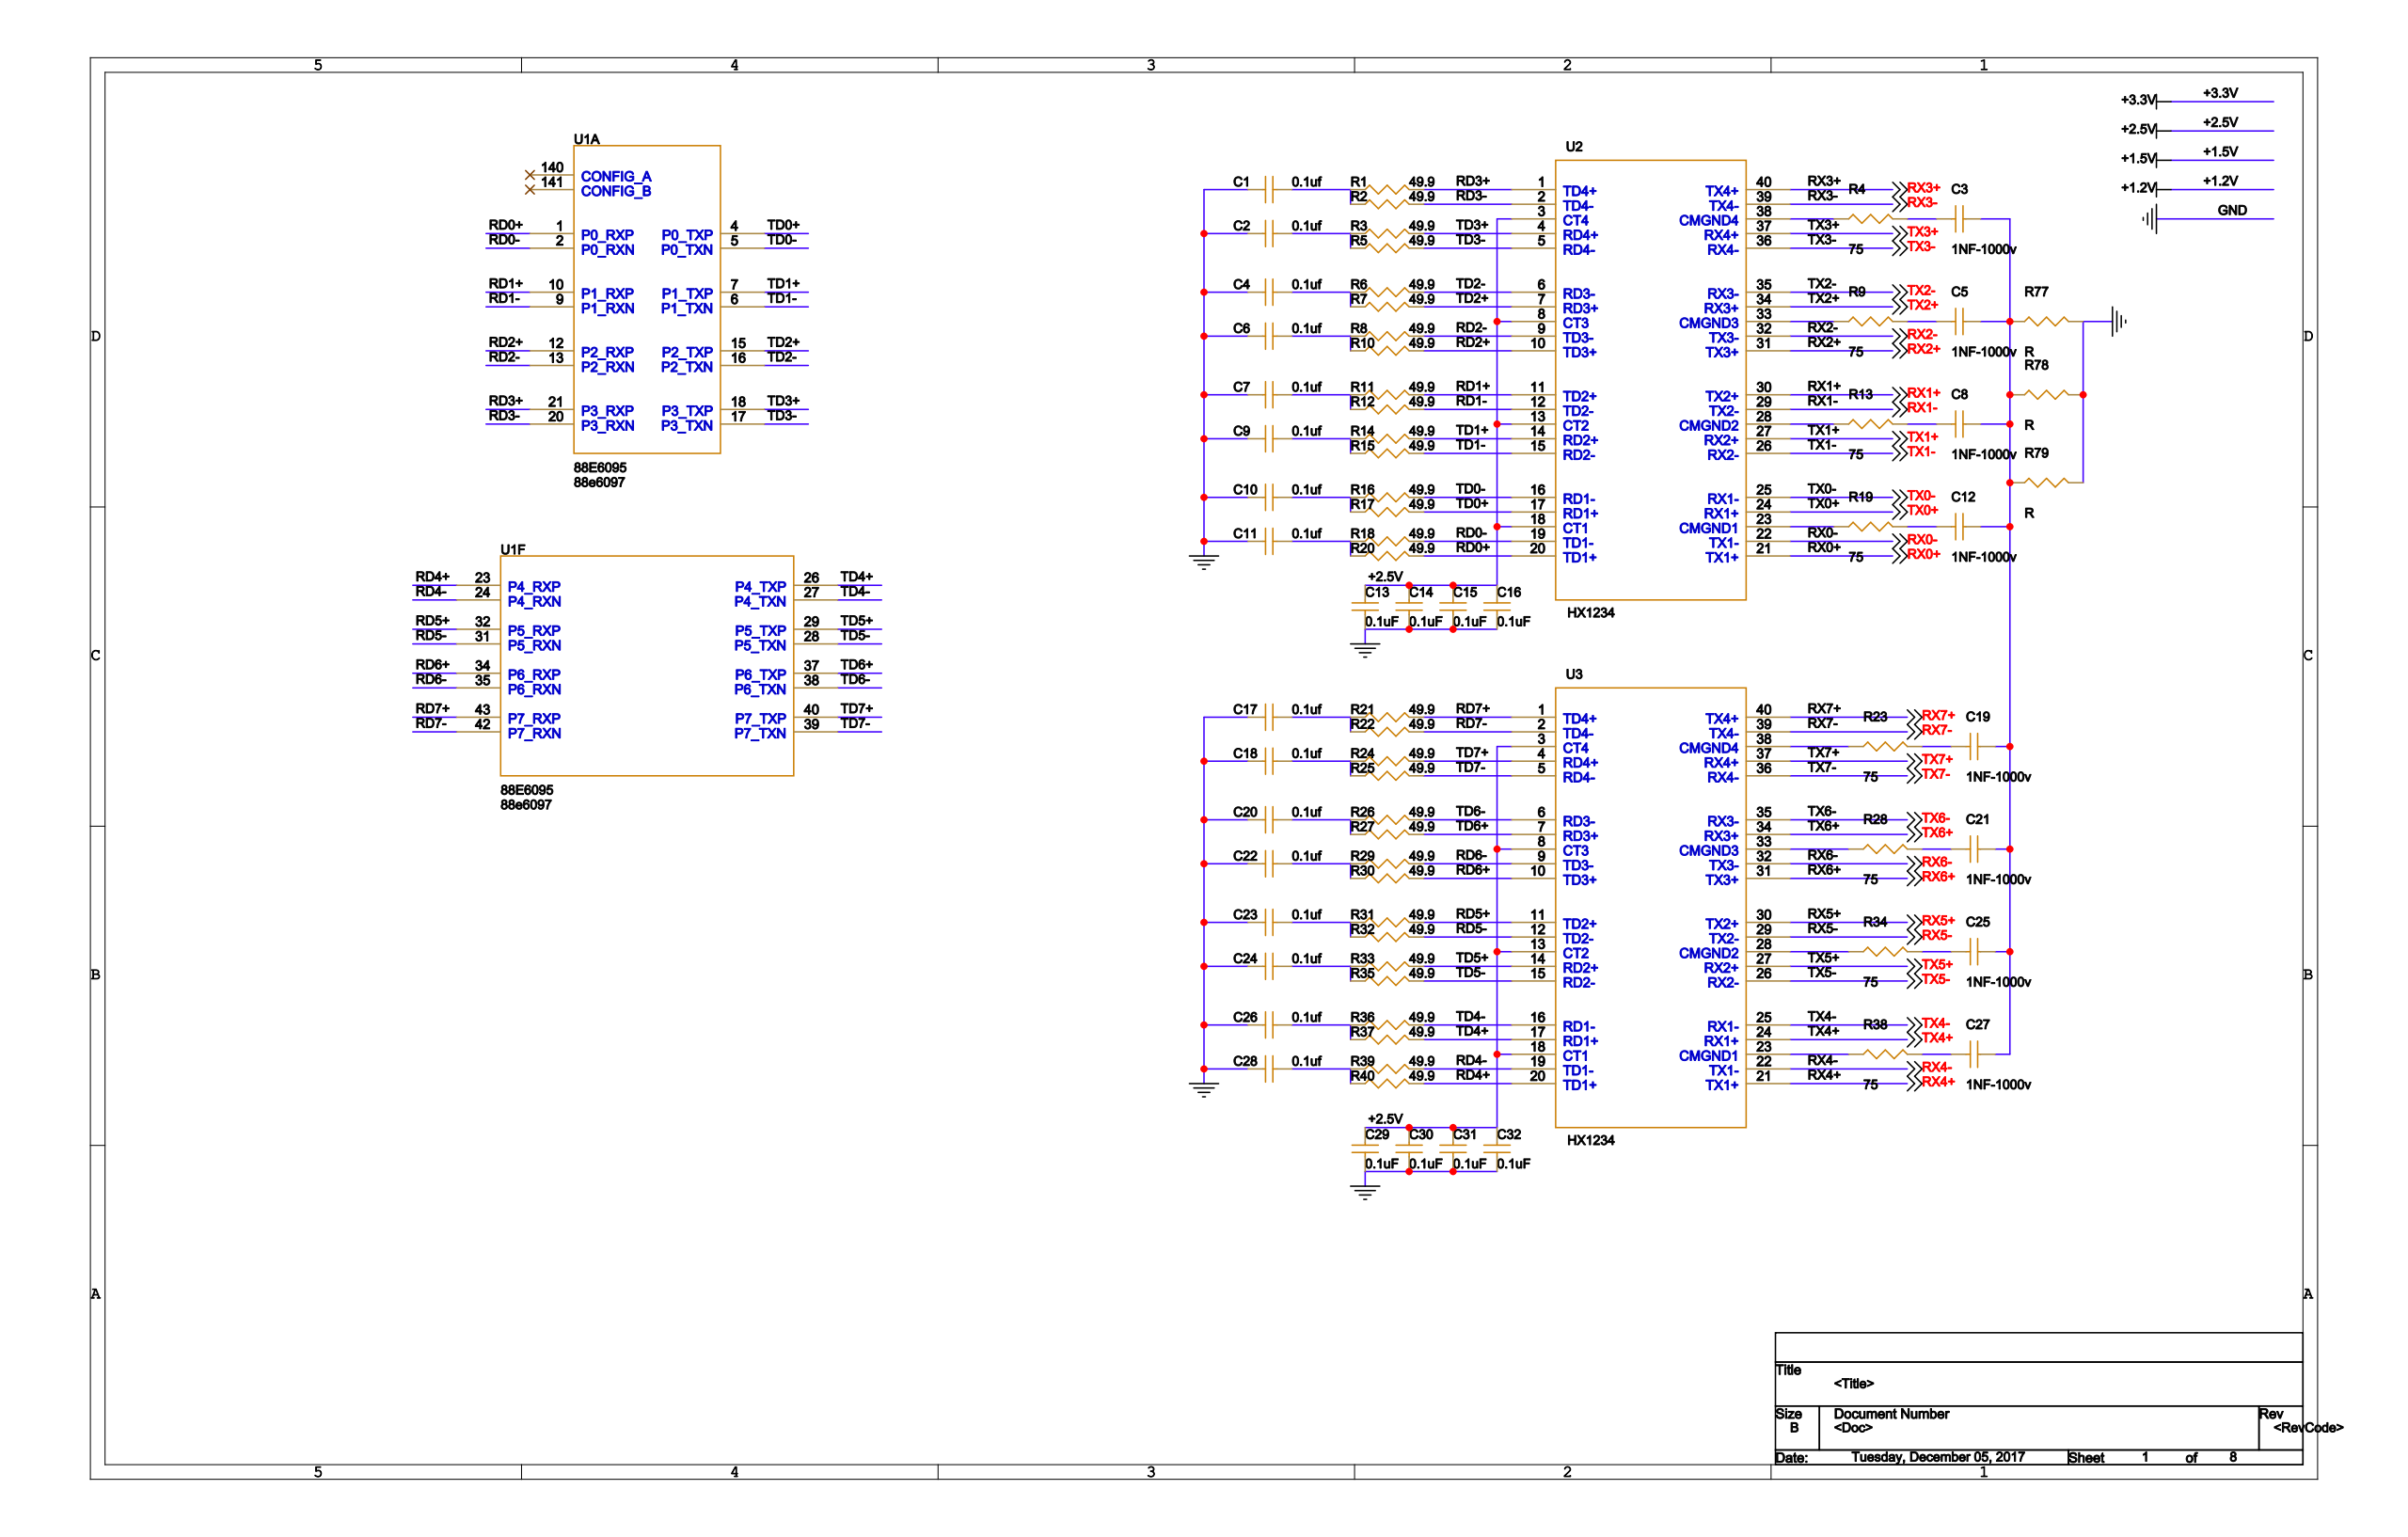Circuit board | Cadence Allegro | 219 parts | 174 nets | one sheet of the schematic
Parts on this sheet (reference | value | footprint):
C1 | 0.1uf | SC0603
C2 | 0.1uf | SC0603
C3 | 1NF-1000v | SC1206
C4 | 0.1uf | SC0603
C5 | 1NF-1000v | SC1206
C6 | 0.1uf | SC0603
C7 | 0.1uf | SC0603
C8 | 1NF-1000v | SC1206
C9 | 0.1uf | SC0603
C10 | 0.1uf | SC0603
C11 | 0.1uf | SC0603
C12 | 1NF-1000v | SC1206
C13 | 0.1uf | SC0603
C14 | 0.1uf | SC0603
C15 | 0.1uf | SC0603
C16 | 0.1uf | SC0603
C17 | 0.1uf | SC0603
C18 | 0.1uf | SC0603
C19 | 1NF-1000v | SC1206
C20 | 0.1uf | SC0603
C21 | 1NF-1000v | SC1206
C22 | 0.1uf | SC0603
C23 | 0.1uf | SC0603
C24 | 0.1uf | SC0603
C25 | 1NF-1000v | SC1206
C26 | 0.1uf | SC0603
C27 | 1NF-1000v | SC1206
C28 | 0.1uf | SC0603
C29 | 0.1uf | SC0603
C30 | 0.1uf | SC0603
C31 | 0.1uf | SC0603
C32 | 0.1uf | SC0603
R1 | 49.9 | SR0603
R2 | 49.9 | SR0603
R3 | 49.9 | SR0603
R4 | 75 | SR0603
R5 | 49.9 | SR0603
R6 | 49.9 | SR0603
R7 | 49.9 | SR0603
R8 | 49.9 | SR0603
R9 | 75 | SR0603
R10 | 49.9 | SR0603
R11 | 49.9 | SR0603
R12 | 49.9 | SR0603
R13 | 75 | SR0603
R14 | 49.9 | SR0603
R15 | 49.9 | SR0603
R16 | 49.9 | SR0603
R17 | 49.9 | SR0603
R18 | 49.9 | SR0603
R19 | 75 | SR0603
R20 | 49.9 | SR0603
R21 | 49.9 | SR0603
R22 | 49.9 | SR0603
R23 | 75 | SR0603
R24 | 49.9 | SR0603
R25 | 49.9 | SR0603
R26 | 49.9 | SR0603
R27 | 49.9 | SR0603
R28 | 75 | SR0603
R29 | 49.9 | SR0603
R30 | 49.9 | SR0603
R31 | 49.9 | SR0603
R32 | 49.9 | SR0603
R33 | 49.9 | SR0603
R34 | 75 | SR0603
R35 | 49.9 | SR0603
R36 | 49.9 | SR0603
R37 | 49.9 | SR0603
R38 | 75 | SR0603
R39 | 49.9 | SR0603
R40 | 49.9 | SR0603
R77 | R | SD1206
R78 | R | SD1206
R79 | R | SD1206
U1 | 88E6095 | 88E6097
U2 | HX1234 | SO-40
U3 | HX1234 | SO-40
Nets of these parts (net: part-pin ...):
N1353026: C3-1 C5-1 C8-1 C12-1 C19-1 C21-1 C25-1 C27-1 R77-1 R78-1 R79-1
GND: C1-1 C2-1 C4-1 C6-1 C7-1 C9-1 C10-1 C11-1 C13-2 C14-2 C15-2 C16-2 C17-1 C18-1 C20-1 C22-1 C23-1 C24-1 C26-1 C28-1 C29-2 C30-2 C31-2 C32-2 R77-2 R78-2 R79-2
RD0-: R18-2 U1-2 U2-19
RD0+: R20-2 U1-1 U2-20
TD0-: R16-2 U1-5 U2-16
TD0+: R17-2 U1-4 U2-17
RD1-: R12-2 U1-9 U2-12
RD1+: R11-2 U1-10 U2-11
TD1-: R15-2 U1-6 U2-15
TD1+: R14-2 U1-7 U2-14
RD2-: R8-2 U1-13 U2-9
RD2+: R10-2 U1-12 U2-10
TD2-: R6-2 U1-16 U2-6
TD2+: R7-2 U1-15 U2-7
RD3-: R2-2 U1-20 U2-2
RD3+: R1-2 U1-21 U2-1
TD3-: R5-2 U1-17 U2-5
TD3+: R3-2 U1-18 U2-4
+2.5V: C13-1 C14-1 C15-1 C16-1 C29-1 C30-1 C31-1 C32-1 U1-11 U1-22 U1-33 U1-44 U2-3 U2-8 U2-13 U2-18 U3-3 U3-8 U3-13 U3-18
+1.5V: U1-55
+1.2V: U1-3 U1-8 U1-14 U1-19 U1-25 U1-30 U1-36
RD4-: R39-2 U1-24 U3-19
RD4+: R40-2 U1-23 U3-20
TD4-: R36-2 U1-27 U3-16
TD4+: R37-2 U1-26 U3-17
RD5-: R32-2 U1-31 U3-12
RD5+: R31-2 U1-32 U3-11
TD5-: R35-2 U1-28 U3-15
TD5+: R33-2 U1-29 U3-14
RD6-: R29-2 U1-35 U3-9
RD6+: R30-2 U1-34 U3-10
TD6-: R26-2 U1-38 U3-6
TD6+: R27-2 U1-37 U3-7
RD7-: R22-2 U1-42 U3-2
RD7+: R21-2 U1-43 U3-1
TD7-: R25-2 U1-39 U3-5
TD7+: R24-2 U1-40 U3-4
N1353184: C6-2 R8-1 R10-1
N1353110: C1-2 R1-1 R2-1
N1354276: C10-2 R16-1 R17-1
N1353356: C11-2 R18-1 R20-1
N1353445: C17-2 R21-1 R22-1
N1354365: C18-2 R24-1 R25-1
N1353821: C2-2 R3-1 R5-1
N1354456: C20-2 R26-1 R27-1
N1353536: C22-2 R29-1 R30-1
N1353629: C23-2 R31-1 R32-1
N1354549: C24-2 R33-1 R35-1
N1354644: C26-2 R36-1 R37-1
N1353724: C28-2 R39-1 R40-1
N1354104: C4-2 R6-1 R7-1
N1353269: C7-2 R11-1 R12-1
N1354189: C9-2 R14-1 R15-1
N1370469: C12-2 R19-2
N1353022: C19-2 R23-2
N1369224: C21-2 R28-2
N1369317: C25-2 R34-2
N1369411: C27-2 R38-2
N1370337: C3-2 R4-2
N1370381: C5-2 R9-2
N1370425: C8-2 R13-2
N1369313: R13-1 U2-28
N1369407: R19-1 U2-23
N1370598: R23-1 U3-38
N1370596: R28-1 U3-33
N1370592: R34-1 U3-28
N1370594: R38-1 U3-23
N1353018: R4-1 U2-38
N1369220: R9-1 U2-33
TX0+: U2-24
TX0-: U2-25
TX1+: U2-27
TX1-: U2-26
TX2+: U2-34
TX2-: U2-35
TX3+: U2-37
TX3-: U2-36
RX0+: U2-21
RX0-: U2-22
RX1+: U2-30
RX1-: U2-29
RX2+: U2-31
RX2-: U2-32
RX3+: U2-40
RX3-: U2-39
TX4+: U3-24
TX4-: U3-25
TX5+: U3-27
TX5-: U3-26
TX6+: U3-34
TX6-: U3-35
TX7+: U3-37
TX7-: U3-36
RX4+: U3-21
RX4-: U3-22
RX5+: U3-30
RX5-: U3-29
RX6+: U3-31
RX6-: U3-32
RX7+: U3-40
RX7-: U3-39